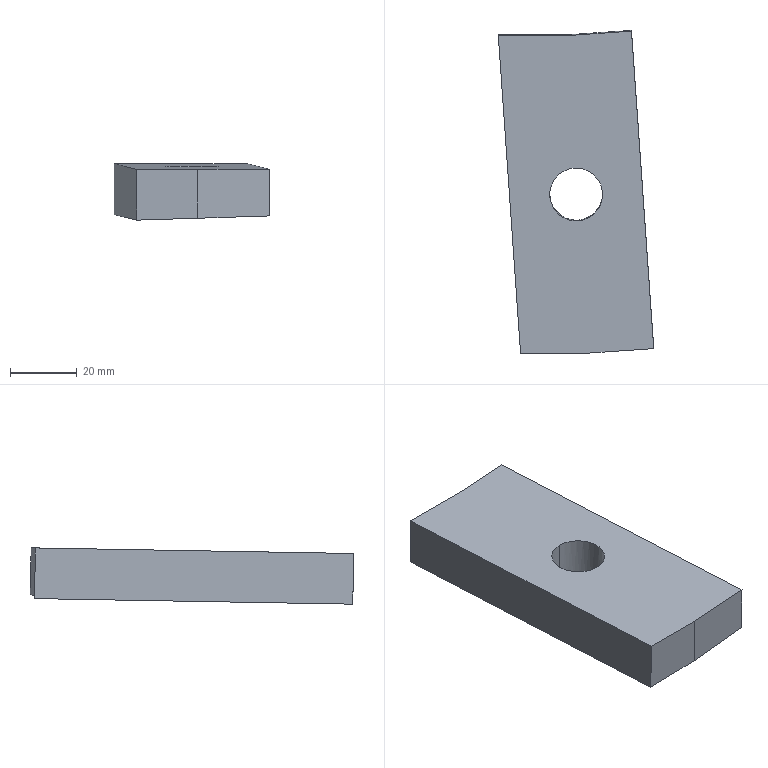Part | SolidWorks | features BaseBody 1 | 1 solid | 10 faces | box 46.683 x 97.109 x 16.906 mm | volume 52978 mm3 | plane 8 | cylinder 2 | commonest cylinder face diameters 15.9 x2
STEP:
#1=CARTESIAN_POINT('',(3.,5.226,-18.523));
#2=VERTEX_POINT('',#1);
#3=CARTESIAN_POINT('',(3.,21.123,-18.21));
#4=VERTEX_POINT('',#3);
#5=CARTESIAN_POINT('',(3.,5.226,-18.523));
#6=CARTESIAN_POINT('',(-12.9,5.235,-19.017));
#7=CARTESIAN_POINT('',(-12.9,21.132,-18.705));
#8=CARTESIAN_POINT('',(3.,21.123,-18.21));
#9=(BOUNDED_CURVE()B_SPLINE_CURVE(3,(#5,#6,#7,#8),.UNSPECIFIED.,.F.,.F.)B_SPLINE_CURVE_WITH_KNOTS((4,4),(1.641,4.782),.UNSPECIFIED.)CURVE()GEOMETRIC_REPRESENTATION_ITEM()RATIONAL_B_SPLINE_CURVE((1.,0.3333,0.3333,1.))REPRESENTATION_ITEM(''));
#10=EDGE_CURVE('',#2,#4,#9,.T.);
#11=ORIENTED_EDGE('',*,*,#10,.T.);
#12=CARTESIAN_POINT('',(3.,20.869,-3.636));
#13=VERTEX_POINT('',#12);
#14=CARTESIAN_POINT('',(3.,21.13,-18.565));
#15=DIRECTION('',(0.,-0.01745,0.9998));
#16=VECTOR('',#15,1000.);
#17=LINE('',#14,#16);
#18=EDGE_CURVE('',#4,#13,#17,.T.);
#19=ORIENTED_EDGE('',*,*,#18,.T.);
#20=CARTESIAN_POINT('',(3.,4.971,-3.914));
#21=VERTEX_POINT('',#20);
#22=CARTESIAN_POINT('',(3.,12.92,-3.775));
#23=DIRECTION('',(0.,-0.01745,0.9998));
#24=DIRECTION('',(0.,-0.9998,-0.01745));
#25=AXIS2_PLACEMENT_3D('',#22,#23,#24);
#26=CIRCLE('',#25,7.95);
#27=EDGE_CURVE('',#13,#21,#26,.T.);
#28=ORIENTED_EDGE('',*,*,#27,.T.);
#29=CARTESIAN_POINT('',(3.,5.232,-18.842));
#30=DIRECTION('',(0.,-0.01745,0.9998));
#31=VECTOR('',#30,1000.);
#32=LINE('',#29,#31);
#33=EDGE_CURVE('',#2,#21,#32,.T.);
#34=ORIENTED_EDGE('',*,*,#33,.F.);
#35=EDGE_LOOP('',(#11,#19,#28,#34));
#36=FACE_OUTER_BOUND('',#35,.T.);
#37=CARTESIAN_POINT('',(3.,13.181,-18.704));
#38=DIRECTION('',(0.,-0.01745,0.9998));
#39=DIRECTION('',(0.,-0.9998,-0.01745));
#40=AXIS2_PLACEMENT_3D('',#37,#38,#39);
#41=CYLINDRICAL_SURFACE('',#40,7.95);
#42=ADVANCED_FACE('',(#36),#41,.F.);
#43=ORIENTED_EDGE('',*,*,#18,.F.);
#44=CARTESIAN_POINT('',(3.,21.123,-18.21));
#45=CARTESIAN_POINT('',(18.9,21.115,-17.716));
#46=CARTESIAN_POINT('',(18.9,5.218,-18.028));
#47=CARTESIAN_POINT('',(3.,5.226,-18.523));
#48=(BOUNDED_CURVE()B_SPLINE_CURVE(3,(#44,#45,#46,#47),.UNSPECIFIED.,.F.,.T.)B_SPLINE_CURVE_WITH_KNOTS((4,4),(4.782,7.924),.UNSPECIFIED.)CURVE()GEOMETRIC_REPRESENTATION_ITEM()RATIONAL_B_SPLINE_CURVE((1.,0.3333,0.3333,1.))REPRESENTATION_ITEM(''));
#49=EDGE_CURVE('',#4,#2,#48,.T.);
#50=ORIENTED_EDGE('',*,*,#49,.T.);
#51=ORIENTED_EDGE('',*,*,#33,.T.);
#52=CARTESIAN_POINT('',(3.,12.92,-3.775));
#53=DIRECTION('',(0.,-0.01745,0.9998));
#54=DIRECTION('',(0.,-0.9998,-0.01745));
#55=AXIS2_PLACEMENT_3D('',#52,#53,#54);
#56=CIRCLE('',#55,7.95);
#57=EDGE_CURVE('',#21,#13,#56,.T.);
#58=ORIENTED_EDGE('',*,*,#57,.T.);
#59=EDGE_LOOP('',(#43,#50,#51,#58));
#60=FACE_OUTER_BOUND('',#59,.T.);
#61=CARTESIAN_POINT('',(3.,13.181,-18.704));
#62=DIRECTION('',(0.,-0.01745,0.9998));
#63=DIRECTION('',(0.,-0.9998,-0.01745));
#64=AXIS2_PLACEMENT_3D('',#61,#62,#63);
#65=CYLINDRICAL_SURFACE('',#64,7.95);
#66=ADVANCED_FACE('',(#60),#65,.F.);
#67=ORIENTED_EDGE('',*,*,#57,.F.);
#68=ORIENTED_EDGE('',*,*,#27,.F.);
#69=EDGE_LOOP('',(#67,#68));
#70=FACE_BOUND('',#69,.T.);
#71=CARTESIAN_POINT('',(-20.395,60.713,-2.941));
#72=VERTEX_POINT('',#71);
#73=CARTESIAN_POINT('',(1.329,60.713,-2.941));
#74=VERTEX_POINT('',#73);
#75=CARTESIAN_POINT('',(2.947,60.713,-2.941));
#76=DIRECTION('',(1.,0.,0.));
#77=VECTOR('',#76,1000.);
#78=LINE('',#75,#77);
#79=EDGE_CURVE('',#72,#74,#78,.T.);
#80=ORIENTED_EDGE('',*,*,#79,.F.);
#81=CARTESIAN_POINT('',(-13.703,-34.872,-4.609));
#82=VERTEX_POINT('',#81);
#83=CARTESIAN_POINT('',(-13.703,-34.872,-4.609));
#84=DIRECTION('',(-0.06982,0.9974,0.01741));
#85=VECTOR('',#84,1000.);
#86=LINE('',#83,#85);
#87=EDGE_CURVE('',#82,#72,#86,.T.);
#88=ORIENTED_EDGE('',*,*,#87,.F.);
#89=CARTESIAN_POINT('',(4.671,-34.872,-4.609));
#90=VERTEX_POINT('',#89);
#91=CARTESIAN_POINT('',(2.947,-34.872,-4.609));
#92=DIRECTION('',(-1.,0.,0.));
#93=VECTOR('',#92,1000.);
#94=LINE('',#91,#93);
#95=EDGE_CURVE('',#90,#82,#94,.T.);
#96=ORIENTED_EDGE('',*,*,#95,.F.);
#97=CARTESIAN_POINT('',(26.289,-33.36,-4.583));
#98=VERTEX_POINT('',#97);
#99=CARTESIAN_POINT('',(26.289,-33.36,-4.583));
#100=DIRECTION('',(-0.9976,-0.06981,-0.001219));
#101=VECTOR('',#100,1000.);
#102=LINE('',#99,#101);
#103=EDGE_CURVE('',#98,#90,#102,.T.);
#104=ORIENTED_EDGE('',*,*,#103,.F.);
#105=CARTESIAN_POINT('',(19.614,61.993,-2.919));
#106=VERTEX_POINT('',#105);
#107=CARTESIAN_POINT('',(19.614,61.993,-2.919));
#108=DIRECTION('',(0.06982,-0.9974,-0.01741));
#109=VECTOR('',#108,1000.);
#110=LINE('',#107,#109);
#111=EDGE_CURVE('',#106,#98,#110,.T.);
#112=ORIENTED_EDGE('',*,*,#111,.F.);
#113=CARTESIAN_POINT('',(1.329,60.713,-2.941));
#114=DIRECTION('',(0.9976,0.06981,0.001219));
#115=VECTOR('',#114,1000.);
#116=LINE('',#113,#115);
#117=EDGE_CURVE('',#74,#106,#116,.T.);
#118=ORIENTED_EDGE('',*,*,#117,.F.);
#119=EDGE_LOOP('',(#80,#88,#96,#104,#112,#118));
#120=FACE_OUTER_BOUND('',#119,.T.);
#121=CARTESIAN_POINT('',(-20.675,-34.872,-4.609));
#122=DIRECTION('',(0.,0.01745,-0.9998));
#123=DIRECTION('',(0.,0.9998,0.01745));
#124=AXIS2_PLACEMENT_3D('',#121,#122,#123);
#125=PLANE('',#124);
#126=ADVANCED_FACE('',(#70,#120),#125,.F.);
#127=ORIENTED_EDGE('',*,*,#10,.F.);
#128=ORIENTED_EDGE('',*,*,#49,.F.);
#129=EDGE_LOOP('',(#127,#128));
#130=FACE_BOUND('',#129,.T.);
#131=CARTESIAN_POINT('',(4.671,-34.617,-19.253));
#132=VERTEX_POINT('',#131);
#133=CARTESIAN_POINT('',(26.289,-33.116,-18.551));
#134=VERTEX_POINT('',#133);
#135=CARTESIAN_POINT('',(4.671,-34.617,-19.253));
#136=DIRECTION('',(0.9971,0.06923,0.03239));
#137=VECTOR('',#136,1000.);
#138=LINE('',#135,#137);
#139=EDGE_CURVE('',#132,#134,#138,.T.);
#140=ORIENTED_EDGE('',*,*,#139,.F.);
#141=CARTESIAN_POINT('',(-13.703,-34.607,-19.825));
#142=VERTEX_POINT('',#141);
#143=CARTESIAN_POINT('',(-13.703,-34.607,-19.825));
#144=DIRECTION('',(0.9995,-0.0005428,0.0311));
#145=VECTOR('',#144,1000.);
#146=LINE('',#143,#145);
#147=EDGE_CURVE('',#142,#132,#146,.T.);
#148=ORIENTED_EDGE('',*,*,#147,.F.);
#149=CARTESIAN_POINT('',(-20.395,60.979,-18.156));
#150=VERTEX_POINT('',#149);
#151=CARTESIAN_POINT('',(-20.395,60.979,-18.156));
#152=DIRECTION('',(0.06982,-0.9974,-0.01741));
#153=VECTOR('',#152,1000.);
#154=LINE('',#151,#153);
#155=EDGE_CURVE('',#150,#142,#154,.T.);
#156=ORIENTED_EDGE('',*,*,#155,.F.);
#157=CARTESIAN_POINT('',(1.329,60.967,-17.48));
#158=VERTEX_POINT('',#157);
#159=CARTESIAN_POINT('',(1.329,60.967,-17.48));
#160=DIRECTION('',(-0.9995,0.0005428,-0.0311));
#161=VECTOR('',#160,1000.);
#162=LINE('',#159,#161);
#163=EDGE_CURVE('',#158,#150,#162,.T.);
#164=ORIENTED_EDGE('',*,*,#163,.F.);
#165=CARTESIAN_POINT('',(19.614,62.236,-16.886));
#166=VERTEX_POINT('',#165);
#167=CARTESIAN_POINT('',(19.614,62.236,-16.886));
#168=DIRECTION('',(-0.9971,-0.06923,-0.03239));
#169=VECTOR('',#168,1000.);
#170=LINE('',#167,#169);
#171=EDGE_CURVE('',#166,#158,#170,.T.);
#172=ORIENTED_EDGE('',*,*,#171,.F.);
#173=CARTESIAN_POINT('',(26.289,-33.116,-18.551));
#174=DIRECTION('',(-0.06982,0.9974,0.01741));
#175=VECTOR('',#174,1000.);
#176=LINE('',#173,#175);
#177=EDGE_CURVE('',#134,#166,#176,.T.);
#178=ORIENTED_EDGE('',*,*,#177,.F.);
#179=EDGE_LOOP('',(#140,#148,#156,#164,#172,#178));
#180=FACE_OUTER_BOUND('',#179,.T.);
#181=CARTESIAN_POINT('',(-20.616,-35.198,-20.051));
#182=DIRECTION('',(-0.0311,-0.01962,0.9993));
#183=DIRECTION('',(0.9995,0.,0.03111));
#184=AXIS2_PLACEMENT_3D('',#181,#182,#183);
#185=PLANE('',#184);
#186=ADVANCED_FACE('',(#130,#180),#185,.F.);
#187=ORIENTED_EDGE('',*,*,#171,.T.);
#188=CARTESIAN_POINT('',(1.329,60.713,-2.941));
#189=DIRECTION('',(0.,0.01745,-0.9998));
#190=VECTOR('',#189,1000.);
#191=LINE('',#188,#190);
#192=EDGE_CURVE('',#74,#158,#191,.T.);
#193=ORIENTED_EDGE('',*,*,#192,.F.);
#194=ORIENTED_EDGE('',*,*,#117,.T.);
#195=CARTESIAN_POINT('',(19.614,62.236,-16.886));
#196=DIRECTION('',(0.,-0.01745,0.9998));
#197=VECTOR('',#196,1000.);
#198=LINE('',#195,#197);
#199=EDGE_CURVE('',#166,#106,#198,.T.);
#200=ORIENTED_EDGE('',*,*,#199,.F.);
#201=EDGE_LOOP('',(#187,#193,#194,#200));
#202=FACE_OUTER_BOUND('',#201,.T.);
#203=CARTESIAN_POINT('',(1.202,60.959,-17.568));
#204=DIRECTION('',(0.06982,-0.9974,-0.01741));
#205=DIRECTION('',(0.9976,0.06983,0.));
#206=AXIS2_PLACEMENT_3D('',#203,#204,#205);
#207=PLANE('',#206);
#208=ADVANCED_FACE('',(#202),#207,.F.);
#209=ORIENTED_EDGE('',*,*,#163,.T.);
#210=CARTESIAN_POINT('',(-20.395,60.847,-10.594));
#211=DIRECTION('',(0.,0.01745,-0.9998));
#212=VECTOR('',#211,1000.);
#213=LINE('',#210,#212);
#214=EDGE_CURVE('',#72,#150,#213,.T.);
#215=ORIENTED_EDGE('',*,*,#214,.F.);
#216=ORIENTED_EDGE('',*,*,#79,.T.);
#217=ORIENTED_EDGE('',*,*,#192,.T.);
#218=EDGE_LOOP('',(#209,#215,#216,#217));
#219=FACE_OUTER_BOUND('',#218,.T.);
#220=CARTESIAN_POINT('',(-20.395,60.713,-2.941));
#221=DIRECTION('',(0.,-0.9998,-0.01745));
#222=DIRECTION('',(0.,0.01745,-0.9998));
#223=AXIS2_PLACEMENT_3D('',#220,#221,#222);
#224=PLANE('',#223);
#225=ADVANCED_FACE('',(#219),#224,.F.);
#226=ORIENTED_EDGE('',*,*,#155,.T.);
#227=CARTESIAN_POINT('',(-13.703,-34.605,-19.916));
#228=DIRECTION('',(0.,0.01745,-0.9998));
#229=VECTOR('',#228,1000.);
#230=LINE('',#227,#229);
#231=EDGE_CURVE('',#82,#142,#230,.T.);
#232=ORIENTED_EDGE('',*,*,#231,.F.);
#233=ORIENTED_EDGE('',*,*,#87,.T.);
#234=ORIENTED_EDGE('',*,*,#214,.T.);
#235=EDGE_LOOP('',(#226,#232,#233,#234));
#236=FACE_OUTER_BOUND('',#235,.T.);
#237=CARTESIAN_POINT('',(-13.644,-35.446,-19.926));
#238=DIRECTION('',(0.9976,0.06981,0.001219));
#239=DIRECTION('',(-0.06981,0.9976,0.));
#240=AXIS2_PLACEMENT_3D('',#237,#238,#239);
#241=PLANE('',#240);
#242=ADVANCED_FACE('',(#236),#241,.F.);
#243=ORIENTED_EDGE('',*,*,#147,.T.);
#244=CARTESIAN_POINT('',(4.671,-34.739,-12.263));
#245=DIRECTION('',(0.,0.01745,-0.9998));
#246=VECTOR('',#245,1000.);
#247=LINE('',#244,#246);
#248=EDGE_CURVE('',#90,#132,#247,.T.);
#249=ORIENTED_EDGE('',*,*,#248,.F.);
#250=ORIENTED_EDGE('',*,*,#95,.T.);
#251=ORIENTED_EDGE('',*,*,#231,.T.);
#252=EDGE_LOOP('',(#243,#249,#250,#251));
#253=FACE_OUTER_BOUND('',#252,.T.);
#254=CARTESIAN_POINT('',(-13.703,-34.605,-19.916));
#255=DIRECTION('',(0.,0.9998,0.01745));
#256=DIRECTION('',(0.,-0.01745,0.9998));
#257=AXIS2_PLACEMENT_3D('',#254,#255,#256);
#258=PLANE('',#257);
#259=ADVANCED_FACE('',(#253),#258,.F.);
#260=ORIENTED_EDGE('',*,*,#139,.T.);
#261=CARTESIAN_POINT('',(26.289,-33.36,-4.583));
#262=DIRECTION('',(0.,0.01745,-0.9998));
#263=VECTOR('',#262,1000.);
#264=LINE('',#261,#263);
#265=EDGE_CURVE('',#98,#134,#264,.T.);
#266=ORIENTED_EDGE('',*,*,#265,.F.);
#267=ORIENTED_EDGE('',*,*,#103,.T.);
#268=ORIENTED_EDGE('',*,*,#248,.T.);
#269=EDGE_LOOP('',(#260,#266,#267,#268));
#270=FACE_OUTER_BOUND('',#269,.T.);
#271=CARTESIAN_POINT('',(26.418,-33.093,-19.341));
#272=DIRECTION('',(-0.06982,0.9974,0.01741));
#273=DIRECTION('',(-0.9976,-0.06983,0.));
#274=AXIS2_PLACEMENT_3D('',#271,#272,#273);
#275=PLANE('',#274);
#276=ADVANCED_FACE('',(#270),#275,.F.);
#277=ORIENTED_EDGE('',*,*,#177,.T.);
#278=ORIENTED_EDGE('',*,*,#199,.T.);
#279=ORIENTED_EDGE('',*,*,#111,.T.);
#280=ORIENTED_EDGE('',*,*,#265,.T.);
#281=EDGE_LOOP('',(#277,#278,#279,#280));
#282=FACE_OUTER_BOUND('',#281,.T.);
#283=CARTESIAN_POINT('',(19.576,62.81,-18.644));
#284=DIRECTION('',(-0.9976,-0.06981,-0.001219));
#285=DIRECTION('',(0.06981,-0.9976,0.));
#286=AXIS2_PLACEMENT_3D('',#283,#284,#285);
#287=PLANE('',#286);
#288=ADVANCED_FACE('',(#282),#287,.F.);
#289=CLOSED_SHELL('',(#42,#66,#126,#186,#208,#225,#242,#259,#276,#288));
#290=MANIFOLD_SOLID_BREP('',#289);
#291=CARTESIAN_POINT('',(0.,0.,0.));
#292=DIRECTION('',(0.,0.,1.));
#293=DIRECTION('',(1.,0.,0.));
#294=AXIS2_PLACEMENT_3D('',#291,#292,#293);
#295=(LENGTH_UNIT()NAMED_UNIT(*)SI_UNIT(.MILLI.,.METRE.));
#296=UNCERTAINTY_MEASURE_WITH_UNIT(LENGTH_MEASURE(0.00001),#295,'','');
#297=(NAMED_UNIT(*)PLANE_ANGLE_UNIT()SI_UNIT($,.RADIAN.));
#298=(NAMED_UNIT(*)SI_UNIT($,.STERADIAN.)SOLID_ANGLE_UNIT());
#299=(GEOMETRIC_REPRESENTATION_CONTEXT(3)GLOBAL_UNCERTAINTY_ASSIGNED_CONTEXT((#296))GLOBAL_UNIT_ASSIGNED_CONTEXT((#295,#297,#298))REPRESENTATION_CONTEXT('',''));
#300=ADVANCED_BREP_SHAPE_REPRESENTATION('',(#290,#294),#299);